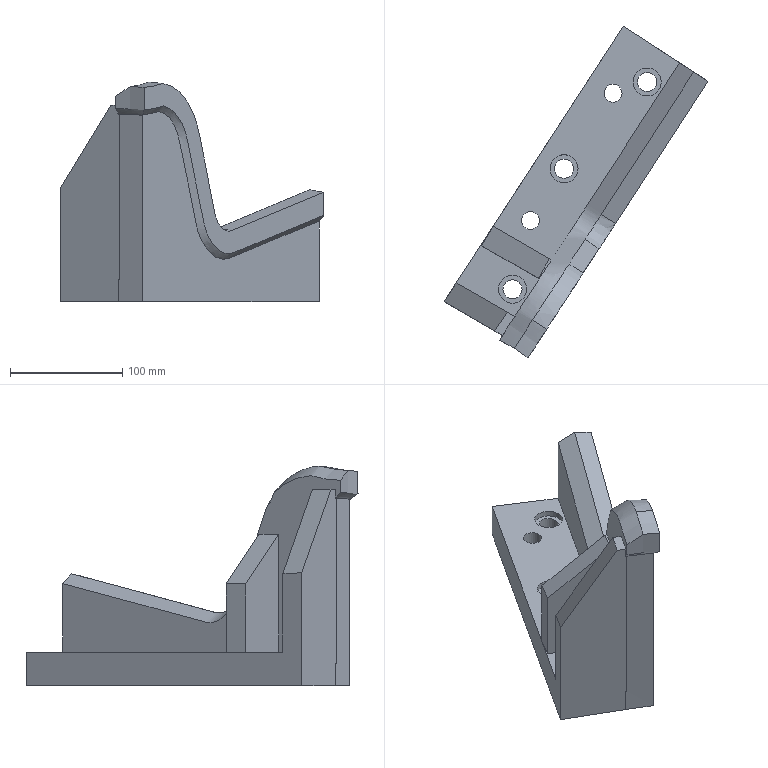Part | NX | features solid 2 | 1 solid | 41 faces | box 234.83 x 295.441 x 195.526 mm | volume 1570629 mm3 | plane 23 | spline 10 | cylinder 8 | commonest cylinder face diameters 17 x3 25 x3 16 x2